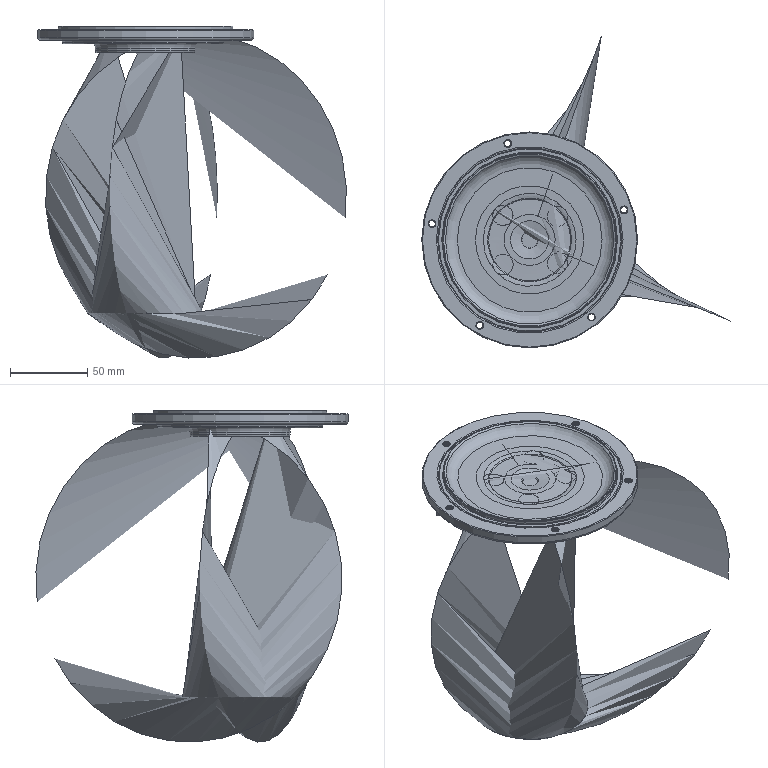NC program | NX | posted with a generic post
Lines 30457 to 31199 of 33119:
(FIXED_CONTOUR_COPY , TOOL : R0.5)
N60900 T02 M6
N60902 G54
N60904 G17 G0 G90 X-60.417 Y-0.5 S9500 M3
N60906 G43 Z30. H2
N60908 Z0.8
N60910 G94 G1 Z-1.85 F1000.
N60912 X-60.416 Y-0.462 Z-2.041
N60914 Y-0.354 Z-2.204
N60916 Y-0.191 Z-2.312
N60918 X-60.415 Y0. Z-2.35
N60920 G2 X-57.918 Y17.189 R60.395 F3500.
N60922 X-52.948 Y29.094 R60.438
N60924 X-28.802 Y53.107 R60.415
N60926 X-17.202 Y57.914 R60.438
N60928 X17.188 Y57.918 R60.415
N60930 X28.789 Y53.115 R60.438
N60932 X53.109 Y28.8 R60.415
N60934 X58.015 Y16.859 R60.438
N60936 X57.917 Y-17.193 R60.415
N60938 X53.109 Y-28.799 R60.438
N60940 X28.807 Y-53.105 R60.415
N60942 X16.865 Y-58.013 R60.438
N60944 X-17.18 Y-57.921 R60.415
N60946 X-29.096 Y-52.947 R60.438
N60948 X-53.105 Y-28.806 R60.415
N60950 X-58.011 Y-16.874 R60.438
N60952 X-60.415 Y0. R60.395
N60954 X34.44 Y49.616 R60.407
N60956 G1 X34.743 Y49.404
N60958 G2 X55.93 Y-22.768 R60.392
N60960 G1 X55.789 Y-23.111 Z-2.351
N60962 G2 X9.994 Y-59.546 R60.382
N60964 G1 X9.628 Y-59.606
N60966 G2 X-35.936 Y-48.513 R60.377
N60968 G1 X-36.234 Y-48.29 Z-2.352
N60970 G2 X-58.454 Y-15.077 R60.369
N60972 G1 X-58.545 Y-14.719
N60974 G2 X-56.71 Y20.677 R60.363
N60976 G1 X-56.583 Y21.024 Z-2.353
N60978 G2 X-34.756 Y49.346 R60.357
N60980 G1 X-34.452 Y49.559
N60982 G2 X-5.546 Y60.098 R60.363
N60984 G1 X-5.178 Y60.131 Z-2.354
N60986 G2 X21.721 Y56.305 R60.344
N60988 G1 X22.066 Y56.171
N60990 G2 X45.946 Y39.123 R60.342
N60992 G1 X46.184 Y38.842 Z-2.355
N60994 G2 X58.047 Y16.483 R60.348
N60996 G1 X58.147 Y16.127
N60998 G2 X59.513 Y-9.951 R60.342
N61000 G1 X59.45 Y-10.317 Z-2.356
N61002 G2 X51.175 Y-31.961 R60.351
N61004 G1 X50.978 Y-32.275
N61006 G2 X35.037 Y-49.116 R60.341
N61008 G1 X34.735 Y-49.33 Z-2.357
N61010 G2 X15.771 Y-58.232 R60.345
N61012 G1 X15.414 Y-58.327
N61014 G2 X-6.655 Y-59.959 R60.328
N61016 G1 X-7.024 Y-59.917 Z-2.358
N61018 G2 X-24.76 Y-55.008 R60.325
N61020 G1 X-25.097 Y-54.856
N61022 G2 X-42.135 Y-43.166 R60.308
N61024 G1 X-42.399 Y-42.907 Z-2.359
N61026 G2 X-53.54 Y-27.783 R60.303
N61028 G1 X-53.708 Y-27.455
N61030 G2 X-59.811 Y-7.795 R60.324
N61032 G1 X-59.857 Y-7.426 Z-2.36
N61034 G2 X-59.291 Y11.06 R60.327
N61036 G1 X-59.222 Y11.423
N61038 G2 X-54.051 Y26.757 R60.325
N61040 G1 X-53.886 Y27.087 Z-2.361
N61042 G2 X-43.417 Y41.858 R60.293
N61044 G1 X-43.159 Y42.124
N61046 G2 X-29.721 Y52.474 R60.292
N61048 G1 X-29.399 Y52.656 Z-2.362
N61050 G2 X-12.87 Y58.915 R60.323
N61052 G1 X-12.507 Y58.993
N61054 G2 X3.341 Y60.21 R60.302
N61056 G1 X3.71 Y60.188 Z-2.363
N61058 G2 X18.568 Y57.37 R60.282
N61060 G1 X18.92 Y57.255
N61062 G2 X34.386 Y49.533 R60.311
N61064 G1 X34.688 Y49.321 Z-2.364
N61066 G2 X45.667 Y39.371 R60.308
N61068 G1 X45.907 Y39.091
N61070 G2 X53.521 Y27.763 R60.276
N61072 G1 X53.69 Y27.435 Z-2.365
N61074 G2 X59.051 Y12.167 R60.307
N61076 G1 X59.125 Y11.805
N61078 G2 X60.261 Y-1.858 R60.286
N61080 G1 X60.249 Y-2.226 Z-2.366
N61082 G2 X58.101 Y-16.09 R60.267
N61084 G1 X58.001 Y-16.446
N61086 G2 X52.639 Y-29.386 R60.307
N61088 G1 X52.458 Y-29.708 Z-2.367
N61090 G2 X44.171 Y-41.025 R60.263
N61092 G1 X43.918 Y-41.296
N61094 G2 X32.87 Y-50.533 R60.277
N61096 G1 X32.559 Y-50.733 Z-2.368
N61098 G2 X22.402 Y-55.963 R60.292
N61100 G1 X22.06 Y-56.099
N61102 G2 X7.035 Y-59.867 R60.274
N61104 G1 X6.665 Y-59.909 Z-2.369
N61106 G2 X-6.28 Y-59.949 R60.304
N61108 G1 X-6.649 Y-59.909
N61110 G2 X-17.847 Y-57.572 R60.259
N61112 G1 X-18.199 Y-57.462 Z-2.37
N61114 G2 X-30.635 Y-51.907 R60.293
N61116 G1 X-30.953 Y-51.718
N61118 G2 X-40.755 Y-44.404 R60.25
N61120 G1 X-41.027 Y-44.152 Z-2.371
N61122 G2 X-49.704 Y-34.087 R60.271
N61124 G1 X-49.912 Y-33.782
N61126 G2 X-54.941 Y-24.775 R60.272
N61128 G1 X-55.091 Y-24.438 Z-2.372
N61130 G2 X-59.239 Y-11.081 R60.276
N61132 G1 X-59.306 Y-10.717
N61134 G2 X-60.265 Y0. R60.254
N61136 G1 X-60.264 Y0.37 Z-2.373
N61138 G2 X-58.876 Y12.86 R60.247
N61140 G1 X-58.796 Y13.22 Z-2.374
N61142 G2 X-55.821 Y22.706 R60.272
N61144 G1 X-55.681 Y23.047
N61146 G2 X-49.079 Y34.966 R60.265
N61148 G1 X-48.863 Y35.267 Z-2.375
N61150 G2 X-42.342 Y42.875 R60.254
N61152 G1 X-42.078 Y43.134
N61154 G2 X-32.546 Y50.712 R60.24
N61156 G1 X-32.234 Y50.911 Z-2.376
N61158 G2 X-24.084 Y55.233 R60.265
N61160 G1 X-23.746 Y55.38
N61162 G2 X-11.043 Y59.234 R60.262
N61164 G1 X-10.678 Y59.3 Z-2.377
N61166 G2 X-1.114 Y60.243 R60.237
N61168 G1 X-0.742 Y60.248
N61170 G2 X11.027 Y59.234 R60.244
N61172 G1 X11.39 Y59.165 Z-2.378
N61174 G2 X19.953 Y56.85 R60.25
N61176 G1 X20.301 Y56.727
N61178 G2 X31.582 Y51.308 R60.265
N61180 G1 X31.895 Y51.113 Z-2.379
N61182 G2 X39.889 Y45.15 R60.224
N61184 G1 X40.167 Y44.903
N61186 G2 X47.723 Y36.77 R60.265
N61188 G1 X47.947 Y36.478 Z-2.38
N61190 G2 X52.781 Y29.043 R60.228
N61192 G1 X52.958 Y28.719
N61194 G2 X56.839 Y19.964 R60.264
N61196 G1 X56.96 Y19.616 Z-2.381
N61198 G2 X59.737 Y7.781 R60.233
N61200 G1 X59.783 Y7.413
N61202 G2 X60.211 Y-1.856 R60.255
N61204 G1 X60.199 Y-2.224 Z-2.382
N61206 G2 X58.853 Y-12.845 R60.217
N61208 G1 X58.773 Y-13.207
N61210 G2 X56.331 Y-21.338 R60.244
N61212 G1 X56.199 Y-21.683 Z-2.383
N61214 G2 X50.893 Y-32.221 R60.249
N61216 G1 X50.694 Y-32.534
N61218 G2 X44.882 Y-40.172 R60.211
N61220 G1 X44.635 Y-40.446 Z-2.384
N61222 G2 X36.469 Y-47.937 R60.25
N61224 G1 X36.174 Y-48.161
N61226 G2 X28.72 Y-52.944 R60.217
N61228 G1 X28.395 Y-53.118 Z-2.385
N61230 G2 X19.271 Y-57.064 R60.251
N61232 G1 X18.921 Y-57.181
N61234 G2 X7.397 Y-59.773 R60.218
N61236 G1 X7.028 Y-59.817 Z-2.386
N61238 G2 X-2.221 Y-60.186 R60.246
N61240 G1 X-2.589 Y-60.172
N61242 G2 X-13.199 Y-58.762 R60.204
N61244 G1 X-13.558 Y-58.68 Z-2.387
N61246 G2 X-21.662 Y-56.194 R60.233
N61248 G1 X-22.005 Y-56.061
N61250 G2 X-32.809 Y-50.501 R60.235
N61252 G1 X-33.119 Y-50.299 Z-2.388
N61254 G2 X-40.721 Y-44.368 R60.2
N61256 G1 X-40.993 Y-44.116
N61258 G2 X-48.595 Y-35.567 R60.229
N61260 G1 X-48.812 Y-35.268 Z-2.389
N61262 G2 X-53.28 Y-28.063 R60.209
N61264 G1 X-53.451 Y-27.736
N61266 G2 X-57.394 Y-18.223 R60.239
N61268 G1 X-57.504 Y-17.871 Z-2.39
N61270 G2 X-59.845 Y-6.674 R60.202
N61272 G1 X-59.885 Y-6.305
N61274 G2 X-60.123 Y3.321 R60.242
N61276 G1 X-60.102 Y3.691 Z-2.391
N61278 G2 X-58.581 Y13.927 R60.19
N61280 G1 X-58.494 Y14.285
N61282 G2 X-55.774 Y22.688 R60.224
N61284 G1 X-55.634 Y23.028 Z-2.392
N61286 G2 X-49.881 Y33.723 R60.218
N61288 G1 X-49.673 Y34.028
N61290 G2 X-43.858 Y41.251 R60.191
N61292 G1 X-43.602 Y41.521 Z-2.393
N61294 G2 X-34.971 Y49.01 R60.209
N61296 G1 X-34.67 Y49.224
N61298 G2 X-27.397 Y53.611 R60.2
N61300 G1 X-27.068 Y53.778 Z-2.394
N61302 G2 X-17.139 Y57.714 R60.226
N61304 G1 X-16.785 Y57.818
N61306 G2 X-5.899 Y59.914 R60.185
N61308 G1 X-5.532 Y59.949 Z-2.395
N61310 G2 X4.439 Y60.038 R60.235
N61312 G1 X4.807 Y60.01
N61314 G2 X14.632 Y58.396 R60.178
N61316 G1 X14.99 Y58.305 Z-2.396
N61318 G2 X23.378 Y55.475 R60.214
N61320 G1 X23.717 Y55.33
N61322 G2 X34.331 Y49.449 R60.202
N61324 G1 X34.633 Y49.238 Z-2.397
N61326 G2 X41.771 Y43.346 R60.183
N61328 G1 X42.038 Y43.086
N61330 G2 X49.427 Y34.357 R60.189
N61332 G1 X49.638 Y34.052 Z-2.398
N61334 G2 X53.933 Y26.731 R60.191
N61336 G1 X54.096 Y26.4
N61338 G2 X58.004 Y16.084 R60.211
N61340 G1 X58.101 Y15.729 Z-2.399
N61342 G2 X59.966 Y5.194 R60.171
N61344 G1 X59.997 Y4.824
N61346 G2 X59.935 Y-5.534 R60.221
N61348 G1 X59.9 Y-5.902 Z-2.4
N61350 G2 X58.198 Y-15.349 R60.168
N61352 G1 X58.103 Y-15.706
N61354 G2 X55.024 Y-24.389 R60.204
N61356 G1 X54.873 Y-24.726 Z-2.401
N61358 G2 X48.776 Y-35.259 R60.185
N61360 G1 X48.559 Y-35.557 Z-2.402
N61362 G2 X42.815 Y-42.296 R60.177
N61364 G1 X42.553 Y-42.56
N61366 G2 X33.738 Y-49.837 R60.172
N61368 G1 X33.432 Y-50.043 Z-2.403
N61370 G2 X26.071 Y-54.241 R60.182
N61372 G1 X25.739 Y-54.399
N61374 G2 X15.015 Y-58.277 R60.197
N61376 G1 X14.657 Y-58.368 Z-2.404
N61378 G2 X4.433 Y-60.015 R60.157
N61380 G1 X4.061 Y-60.041
N61382 G2 X-6.638 Y-59.81 R60.204
N61384 G1 X-7.005 Y-59.768 Z-2.405
N61386 G2 X-16.049 Y-57.996 R60.157
N61388 G1 X-16.404 Y-57.896
N61390 G2 X-25.037 Y-54.718 R60.192
N61392 G1 X-25.371 Y-54.564 Z-2.406
N61394 G2 X-35.821 Y-48.349 R60.169
N61396 G1 X-36.118 Y-48.128
N61398 G2 X-42.814 Y-42.28 R60.171
N61400 G1 X-43.072 Y-42.017 Z-2.407
N61402 G2 X-50.035 Y-33.42 R60.155
N61404 G1 X-50.239 Y-33.113
N61406 G2 X-54.387 Y-25.735 R60.171
N61408 G1 X-54.544 Y-25.402 Z-2.408
N61410 G2 X-58.353 Y-14.663 R60.184
N61412 G1 X-58.442 Y-14.305
N61414 G2 X-60.027 Y-4.078 R60.144
N61416 G1 X-60.051 Y-3.707 Z-2.409
N61418 G2 X-59.754 Y7.012 R60.189
N61420 G1 X-59.71 Y7.38
N61422 G2 X-57.882 Y16.409 R60.146
N61424 G1 X-57.781 Y16.763 Z-2.41
N61426 G2 X-54.396 Y25.7 R60.181
N61428 G1 X-54.238 Y26.032
N61430 G2 X-47.899 Y36.4 R60.154
N61432 G1 X-47.674 Y36.694 Z-2.411
N61434 G2 X-41.479 Y43.572 R60.168
N61436 G1 X-41.212 Y43.825
N61438 G2 X-32.493 Y50.627 R60.138
N61440 G1 X-32.181 Y50.826 Z-2.412
N61442 G2 X-24.718 Y54.843 R60.163
N61444 G1 X-24.381 Y54.994
N61446 G2 X-13.196 Y58.689 R60.167
N61448 G1 X-12.836 Y58.769 Z-2.413
N61450 G2 X-3.325 Y60.061 R60.131
N61452 G1 X-2.957 Y60.08
N61454 G2 X8.097 Y59.604 R60.167
N61456 G1 X8.462 Y59.554 Z-2.414
N61458 G2 X17.112 Y57.665 R60.137
N61460 G1 X17.466 Y57.559
N61462 G2 X26.706 Y53.895 R60.169
N61464 G1 X27.035 Y53.731 Z-2.415
N61466 G2 X36.977 Y47.439 R60.137
N61468 G1 X37.268 Y47.211
N61470 G2 X44.078 Y40.924 R60.164
N61472 G1 X44.328 Y40.652 Z-2.416
N61474 G2 X50.817 Y32.173 R60.124
N61476 G1 X51.013 Y31.86
N61478 G2 X55.131 Y24.037 R60.152
N61480 G1 X55.277 Y23.7 Z-2.417
N61482 G2 X58.83 Y12.493 R60.152
N61484 G1 X58.906 Y12.132
N61486 G2 X60.085 Y2.595 R60.121
N61488 G1 X60.099 Y2.223 Z-2.418
N61490 G2 X59.488 Y-8.823 R60.148
N61492 G1 X59.433 Y-9.188
N61494 G2 X57.438 Y-17.818 R60.128
N61496 G1 X57.327 Y-18.17 Z-2.419
N61498 G2 X53.382 Y-27.69 R60.156
N61500 G1 X53.211 Y-28.017
N61502 G2 X46.95 Y-37.575 R60.121
N61504 G1 X46.719 Y-37.862 Z-2.42
N61506 G2 X40.105 Y-44.807 R60.161
N61508 G1 X39.83 Y-45.051
N61510 G2 X31.543 Y-51.195 R60.111
N61512 G1 X31.228 Y-51.387 Z-2.421
N61514 G2 X23.366 Y-55.405 R60.142
N61516 G1 X23.026 Y-55.547
N61518 G2 X11.401 Y-59.039 R60.136
N61520 G1 X11.038 Y-59.107 Z-2.422
N61522 G2 X1.835 Y-60.1 R60.111
N61524 G1 X1.466 Y-60.11
N61526 G2 X-9.922 Y-59.302 R60.128
N61528 G1 X-10.286 Y-59.24 Z-2.423
N61530 G2 X-18.505 Y-57.207 R60.119
N61532 G1 X-18.855 Y-57.092
N61534 G2 X-28.639 Y-52.865 R60.143
N61536 G1 X-28.963 Y-52.688 Z-2.424
N61538 G2 X-38.129 Y-46.485 R60.106
N61540 G1 X-38.415 Y-46.249
N61542 G2 X-45.523 Y-39.271 R60.151
N61544 G1 X-45.763 Y-38.991 Z-2.425
N61546 G2 X-51.569 Y-30.903 R60.098
N61548 G1 X-51.757 Y-30.587
N61550 G2 X-55.674 Y-22.684 R60.132
N61552 G1 X-55.812 Y-22.343 Z-2.426
N61554 G2 X-59.16 Y-10.684 R60.121
N61556 G1 X-59.224 Y-10.321
N61558 G2 X-60.105 Y-1.104 R60.102
N61560 G1 X-60.111 Y-0.736 Z-2.427
N61562 G2 X-59.162 Y10.657 R60.109
N61564 G1 X-59.095 Y11.02
N61566 G2 X-56.962 Y19.205 R60.11
N61568 G1 X-56.844 Y19.553 Z-2.428
N61570 G2 X-52.499 Y29.277 R60.13
N61572 G1 X-52.319 Y29.598
N61574 G2 X-46.245 Y38.4 R60.092
N61576 G1 X-46.007 Y38.685 Z-2.429
N61578 G2 X-38.699 Y45.994 R60.138
N61580 G1 X-38.416 Y46.23 Z-2.43
N61582 G2 X-30.581 Y51.746 R60.087
N61584 G1 X-30.263 Y51.933
N61586 G2 X-21.983 Y55.941 R60.121
N61588 G1 X-21.64 Y56.075 Z-2.431
N61590 G2 X-9.922 Y59.28 R60.105
N61592 G1 X-9.557 Y59.34
N61594 G2 X-0.74 Y60.098 R60.093
N61596 G1 X-0.369 Y60.102 Z-2.432
N61598 G2 X10.999 Y59.086 R60.093
N61600 G1 X11.362 Y59.018
N61602 G2 X19.555 Y56.83 R60.099
N61604 G1 X19.903 Y56.709 Z-2.433
N61606 G2 X29.926 Y52.118 R60.116
N61608 G1 X30.244 Y51.934
N61610 G2 X38.953 Y45.764 R60.078
N61612 G1 X39.234 Y45.523 Z-2.434
N61614 G2 X46.693 Y37.833 R60.122
N61616 G1 X46.923 Y37.546
N61618 G2 X52.108 Y29.936 R60.077
N61620 G1 X52.29 Y29.615 Z-2.435
N61622 G2 X56.194 Y21.293 R60.109
N61624 G1 X56.323 Y20.949
N61626 G2 X59.38 Y9.219 R60.09
N61628 G1 X59.436 Y8.854 Z-2.436
N61630 G2 X60.089 Y-0.378 R60.089
N61632 G1 X60.086 Y-0.747
N61634 G2 X58.933 Y-11.728 R60.075
N61636 G1 X58.86 Y-12.09 Z-2.437
N61638 G2 X56.573 Y-20.248 R60.089
N61640 G1 X56.448 Y-20.594
N61642 G2 X51.541 Y-30.885 R60.101
N61644 G1 X51.35 Y-31.201 Z-2.438
N61646 G2 X45.258 Y-39.52 R60.064
N61648 G1 X45.015 Y-39.797
N61650 G2 X37.255 Y-47.139 R60.106
N61652 G1 X36.964 Y-47.367 Z-2.439
N61654 G2 X29.293 Y-52.457 R60.066
N61656 G1 X28.971 Y-52.635
N61658 G2 X20.262 Y-56.561 R60.098
N61660 G1 X19.915 Y-56.684 Z-2.44
N61662 G2 X8.476 Y-59.478 R60.074
N61664 G1 X8.11 Y-59.529
N61666 G2 X-1.113 Y-60.067 R60.083
N61668 G1 X-1.48 Y-60.059 Z-2.441
N61670 G2 X-12.446 Y-58.773 R60.059
N61672 G1 X-12.806 Y-58.695
N61674 G2 X-21.266 Y-56.185 R60.081
N61676 G1 X-21.609 Y-56.054 Z-2.442
N61678 G2 X-32.111 Y-50.771 R60.085
N61680 G1 X-32.422 Y-50.573
N61682 G2 X-40.07 Y-44.756 R60.052
N61684 G1 X-40.345 Y-44.507 Z-2.443
N61686 G2 X-47.811 Y-36.367 R60.086
N61688 G1 X-48.034 Y-36.073
N61690 G2 X-52.801 Y-28.641 R60.057
N61692 G1 X-52.976 Y-28.318 Z-2.444
N61694 G2 X-56.91 Y-19.221 R60.086
N61696 G1 X-57.026 Y-18.873
N61698 G2 X-59.61 Y-7.387 R60.057
N61700 G1 X-59.655 Y-7.02 Z-2.445
N61702 G2 X-60.01 Y2.577 R60.083
N61704 G1 X-59.993 Y2.945
N61706 G2 X-58.519 Y13.532 R60.044
N61708 G1 X-58.435 Y13.89 Z-2.446
N61710 G2 X-55.772 Y22.292 R60.072
N61712 G1 X-55.635 Y22.633
N61714 G2 X-50.163 Y33.03 R60.069
N61716 G1 X-49.959 Y33.337 Z-2.447
N61718 G2 X-44.002 Y40.877 R60.042
N61720 G1 X-43.749 Y41.148
N61722 G2 X-35.482 Y48.456 R60.063
N61724 G1 X-35.184 Y48.673 Z-2.448
N61726 G2 X-27.657 Y53.309 R60.049
N61728 G1 X-27.329 Y53.478
N61730 G2 X-17.799 Y57.357 R60.074
N61732 G1 X-17.447 Y57.465 Z-2.449
N61734 G2 X-6.251 Y59.728 R60.04
N61736 G1 X-5.885 Y59.765
N61738 G2 X4.06 Y59.915 R60.08
N61740 G1 X4.427 Y59.889 Z-2.45
N61742 G2 X14.237 Y58.339 R60.031
N61744 G1 X14.595 Y58.25
N61746 G2 X22.98 Y55.479 R60.062
N61748 G1 X23.32 Y55.337 Z-2.451
N61750 G2 X33.642 Y49.739 R60.053
N61752 G1 X33.946 Y49.532
N61754 G2 X41.129 Y43.749 R60.031
N61756 G1 X41.399 Y43.494 Z-2.452
N61758 G2 X48.664 Y35.175 R60.047
N61760 G1 X48.879 Y34.875
N61762 G2 X53.468 Y27.322 R60.038
N61764 G1 X53.634 Y26.994 Z-2.453
N61766 G2 X57.451 Y17.451 R60.06
N61768 G1 X57.556 Y17.099
N61770 G2 X59.712 Y6.282 R60.027
N61772 G1 X59.749 Y5.914 Z-2.454
N61774 G2 X59.903 Y-4.05 R60.065
N61776 G1 X59.877 Y-4.417
N61778 G2 X58.326 Y-14.238 R60.019
N61780 G1 X58.237 Y-14.596 Z-2.455
N61782 G2 X55.467 Y-22.976 R60.049
N61784 G1 X55.325 Y-23.316
N61786 G2 X49.713 Y-33.659 R60.041
N61788 G1 X49.505 Y-33.964 Z-2.456
N61790 G2 X43.735 Y-41.126 R60.018
N61792 G1 X43.481 Y-41.394
N61794 G2 X35.164 Y-48.657 R60.035
N61796 G1 X34.864 Y-48.872 Z-2.457
N61798 G2 X27.323 Y-53.453 R60.025
N61800 G1 X26.995 Y-53.62
N61802 G2 X17.452 Y-57.437 R60.048
N61804 G1 X17.1 Y-57.543 Z-2.458
N61806 G2 X6.266 Y-59.701 R60.015
N61808 G1 X5.897 Y-59.738
N61810 G2 X-4.048 Y-59.891 R60.053
N61812 G1 X-4.415 Y-59.865 Z-2.459
N61814 G2 X-14.229 Y-58.315 R60.006
N61816 G1 X-14.586 Y-58.227 Z-2.46
N61818 G2 X-22.956 Y-55.461 R60.036
N61820 G1 X-23.295 Y-55.32
N61822 G2 X-33.627 Y-49.719 R60.029
N61824 G1 X-33.932 Y-49.512 Z-2.461
N61826 G2 X-41.126 Y-43.719 R60.006
N61828 G1 X-41.393 Y-43.465
N61830 G2 X-48.649 Y-35.152 R60.023
N61832 G1 X-48.864 Y-34.853 Z-2.462
N61834 G2 X-53.442 Y-27.317 R60.013
N61836 G1 X-53.608 Y-26.99
N61838 G2 X-57.423 Y-17.455 R60.035
N61840 G1 X-57.529 Y-17.103 Z-2.463
N61842 G2 X-59.687 Y-6.278 R60.003
N61844 G1 X-59.725 Y-5.91
N61846 G2 X-59.878 Y4.049 R60.04
N61848 G1 X-59.852 Y4.418 Z-2.464
N61850 G2 X-58.301 Y14.236 R59.994
N61852 G1 X-58.212 Y14.592
N61854 G2 X-55.449 Y22.954 R60.024
N61856 G1 X-55.307 Y23.293 Z-2.465
N61858 G2 X-49.711 Y33.616 R60.016
N61860 G1 X-49.504 Y33.921
N61862 G2 X-43.712 Y41.114 R59.994
N61864 G1 X-43.458 Y41.382 Z-2.466
N61866 G2 X-35.154 Y48.633 R60.01
N61868 G1 X-34.855 Y48.847
N61870 G2 X-27.307 Y53.433 R60.001
N61872 G1 X-26.979 Y53.6 Z-2.467
N61874 G2 X-17.432 Y57.417 R60.023
N61876 G1 X-17.08 Y57.523
N61878 G2 X-6.246 Y59.678 R59.99
N61880 G1 X-5.88 Y59.715 Z-2.468
N61882 G2 X4.056 Y59.865 R60.028
N61884 G1 X4.423 Y59.839
N61886 G2 X14.225 Y58.29 R59.982
N61888 G1 X14.582 Y58.202 Z-2.469
N61890 G2 X23.3 Y55.291 R60.011
N61892 G1 X23.639 Y55.147
N61894 G2 X33.919 Y49.49 R60.002
N61896 G1 X34.222 Y49.281 Z-2.47
N61898 G2 X41.365 Y43.458 R59.984
N61900 G1 X41.633 Y43.201
N61902 G2 X48.838 Y34.846 R59.994
N61904 G1 X49.052 Y34.546 Z-2.471
N61906 G2 X53.589 Y26.971 R59.99
N61908 G1 X53.754 Y26.643
N61910 G2 X57.612 Y16.732 R60.009
N61912 G1 X57.713 Y16.379 Z-2.472
N61914 G2 X59.735 Y5.54 R59.976
N61916 G1 X59.768 Y5.172
N61918 G2 X59.768 Y-5.148 R60.016
N61920 G1 X59.736 Y-5.515 Z-2.473
N61922 G2 X58.098 Y-14.941 R59.971
N61924 G1 X58.005 Y-15.297
N61926 G2 X54.989 Y-23.972 R60.
N61928 G1 X54.841 Y-24.309 Z-2.474
N61930 G2 X49.043 Y-34.541 R59.987
N61932 G1 X48.829 Y-34.842
N61934 G2 X42.932 Y-41.892 R59.975
N61936 G1 X42.673 Y-42.156 Z-2.475
N61938 G2 X34.234 Y-49.255 R59.976
N61940 G1 X33.931 Y-49.464
N61942 G2 X26.314 Y-53.901 R59.98
N61944 G1 X25.984 Y-54.061 Z-2.476
N61946 G2 X15.67 Y-57.897 R59.995
N61948 G1 X15.315 Y-57.992
N61950 G2 X4.786 Y-59.787 R59.962
N61952 G1 X4.417 Y-59.816 Z-2.477
N61954 G2 X-5.881 Y-59.688 R60.002
N61956 G1 X-6.248 Y-59.651
N61958 G2 X-15.641 Y-57.9 R59.96
N61960 G1 X-15.996 Y-57.803 Z-2.478
N61962 G2 X-24.957 Y-54.535 R59.989
N61964 G1 X-25.291 Y-54.381
N61966 G2 X-35.409 Y-48.404 R59.971
N61968 G1 X-35.706 Y-48.185 Z-2.479
N61970 G2 X-42.671 Y-42.14 R59.969
N61972 G1 X-42.928 Y-41.878
N61974 G2 X-49.868 Y-33.311 R59.958
N61976 G1 X-50.071 Y-33.004 Z-2.48
N61978 G2 X-54.363 Y-25.315 R59.971
N61980 G1 X-54.517 Y-24.982
N61982 G2 X-58.161 Y-14.607 R59.981
N61984 G1 X-58.25 Y-14.25 Z-2.481
N61986 G2 X-59.828 Y-4.061 R59.949
N61988 G1 X-59.852 Y-3.692
N61990 G2 X-59.556 Y6.987 R59.985
N61992 G1 X-59.512 Y7.353 Z-2.482
N61994 G2 X-57.69 Y16.353 R59.949
N61996 G1 X-57.589 Y16.706
N61998 G2 X-54.214 Y25.619 R59.978
N62000 G1 X-54.056 Y25.95 Z-2.483
N62002 G2 X-47.958 Y35.99 R59.956
N62004 G1 X-47.736 Y36.284
N62006 G2 X-41.607 Y43.174 R59.963
N62008 G1 X-41.342 Y43.427 Z-2.484
N62010 G2 X-32.695 Y50.259 R59.943
N62012 G1 X-32.385 Y50.459
N62014 G2 X-24.635 Y54.661 R59.961
N62016 G1 X-24.3 Y54.811 Z-2.485
N62018 G2 X-13.509 Y58.413 R59.966
N62020 G1 X-13.15 Y58.495
N62022 G2 X-3.313 Y59.862 R59.935
N62024 G1 X-2.946 Y59.881 Z-2.486
N62026 G2 X8.07 Y59.406 R59.965
N62028 G1 X8.434 Y59.356
N62030 G2 X17.407 Y57.368 R59.94
N62032 G1 X17.758 Y57.26 Z-2.487
N62034 G2 X26.947 Y53.552 R59.966
N62036 G1 X27.274 Y53.386
N62038 G2 X36.859 Y47.277 R59.939
N62040 G1 X37.149 Y47.05 Z-2.488
N62042 G2 X44.179 Y40.519 R59.963
N62044 G1 X44.427 Y40.247
N62046 G2 X50.647 Y32.066 R59.928
N62048 G1 X50.843 Y31.755 Z-2.489
N62050 G2 X54.948 Y23.957 R59.951
N62052 G1 X55.094 Y23.62 Z-2.49
N62054 G2 X58.559 Y12.804 R59.951
N62056 G1 X58.636 Y12.445
N62058 G2 X59.868 Y2.954 R59.924
N62060 G1 X59.885 Y2.584 Z-2.491
N62062 G2 X59.344 Y-8.43 R59.95
N62064 G1 X59.291 Y-8.794
N62066 G2 X57.355 Y-17.406 R59.929
N62068 G1 X57.247 Y-17.757 Z-2.492
N62070 G2 X53.539 Y-26.945 R59.953
N62072 G1 X53.372 Y-27.272
N62074 G2 X47.249 Y-36.875 R59.926
N62076 G1 X47.022 Y-37.163 Z-2.493
N62078 G2 X40.517 Y-44.164 R59.951
N62080 G1 X40.245 Y-44.412
N62082 G2 X32.062 Y-50.636 R59.915
N62084 G1 X31.751 Y-50.831 Z-2.494
N62086 G2 X23.96 Y-54.933 R59.938
N62088 G1 X23.623 Y-55.079
N62090 G2 X12.799 Y-58.547 R59.939
N62092 G1 X12.44 Y-58.624 Z-2.495
N62094 G2 X2.936 Y-59.856 R59.911
N62096 G1 X2.567 Y-59.873
N62098 G2 X-8.435 Y-59.33 R59.937
N62100 G1 X-8.799 Y-59.277 Z-2.496
N62102 G2 X-17.744 Y-57.238 R59.917
N62104 G1 X-18.095 Y-57.128
N62106 G2 X-27.576 Y-53.202 R59.94
N62108 G1 X-27.901 Y-53.032 Z-2.497
N62110 G2 X-37.142 Y-47.024 R59.912
N62112 G1 X-37.431 Y-46.794
N62114 G2 X-44.399 Y-40.241 R59.94
N62116 G1 X-44.644 Y-39.968 Z-2.498
N62118 G2 X-50.822 Y-31.741 R59.903
N62120 G1 X-51.016 Y-31.429
N62122 G2 X-55.067 Y-23.62 R59.927
N62124 G1 X-55.21 Y-23.283 Z-2.499
N62126 G2 X-58.61 Y-12.446 R59.925
N62128 G1 X-58.686 Y-12.086
N62130 G2 X-59.86 Y-2.579 R59.9
N62132 G1 X-59.875 Y-2.209 Z-2.5
N62134 G2 X-59.264 Y8.805 R59.922
N62136 G1 X-59.209 Y9.169
N62138 G2 X-57.225 Y17.746 R59.905
N62140 G1 X-57.115 Y18.096 Z-2.501
N62142 G2 X-53.191 Y27.57 R59.927
N62144 G1 X-53.021 Y27.895
N62146 G2 X-47.018 Y37.129 R59.9
N62148 G1 X-46.788 Y37.418 Z-2.502
N62150 G2 X-40.233 Y44.389 R59.927
N62152 G1 X-39.96 Y44.635
N62154 G2 X-31.737 Y50.81 R59.89
N62156 G1 X-31.424 Y51.004 Z-2.503
N62158 G2 X-23.269 Y55.202 R59.915
N62160 G1 X-22.93 Y55.344
N62162 G2 X-11.698 Y58.751 R59.911
N62164 G1 X-11.337 Y58.822 Z-2.504
N62166 G2 X-1.842 Y59.875 R59.889
N62168 G1 X-1.474 Y59.885
N62170 G2 X9.515 Y59.141 R59.903
N62172 G1 X9.878 Y59.082 Z-2.505
N62174 G2 X18.444 Y56.99 R59.895
N62176 G1 X18.793 Y56.876
N62178 G2 X28.226 Y52.831 R59.915
N62180 G1 X28.549 Y52.658 Z-2.506
N62182 G2 X37.694 Y46.55 R59.885
N62184 G1 X37.979 Y46.317
N62186 G2 X45.121 Y39.391 R59.919
N62188 G1 X45.361 Y39.114 Z-2.507
N62190 G2 X51.186 Y31.103 R59.878
N62192 G1 X51.376 Y30.788
N62194 G2 X55.472 Y22.585 R59.904
N62196 G1 X55.609 Y22.245 Z-2.508
N62198 G2 X58.875 Y10.993 R59.896
N62200 G1 X58.941 Y10.632
N62202 G2 X59.873 Y1.472 R59.879
N62204 G1 X59.88 Y1.102 Z-2.509
N62206 G2 X59.069 Y-9.877 R59.888
N62208 G1 X59.007 Y-10.24
N62210 G2 X56.863 Y-18.791 R59.884
N62212 G1 X56.747 Y-19.14 Z-2.51
N62214 G2 X52.467 Y-28.872 R59.902
N62216 G1 X52.289 Y-29.193
N62218 G2 X46.293 Y-37.989 R59.871
N62220 G1 X46.059 Y-38.272 Z-2.511
N62222 G2 X39.113 Y-45.346 R59.908
N62224 G1 X38.834 Y-45.585
N62226 G2 X30.785 Y-51.363 R59.866
N62228 G1 X30.469 Y-51.551 Z-2.512
N62230 G2 X22.248 Y-55.595 R59.892
N62232 G1 X21.907 Y-55.73
N62234 G2 X10.624 Y-58.93 R59.882
N62236 G1 X10.261 Y-58.994 Z-2.513
N62238 G2 X1.095 Y-59.868 R59.867
N62240 G1 X0.727 Y-59.874
N62242 G2 X-10.242 Y-58.994 R59.874
N62244 G1 X-10.603 Y-58.93 Z-2.514
N62246 G2 X-19.126 Y-56.739 R59.873
N62248 G1 X-19.473 Y-56.62
N62250 G2 X-29.169 Y-52.288 R59.888
N62252 G1 X-29.489 Y-52.108 Z-2.515
N62254 G2 X-38.258 Y-46.055 R59.859
N62256 G1 X-38.541 Y-45.818
N62258 G2 X-45.811 Y-38.547 R59.895
N62260 G1 X-46.047 Y-38.265 Z-2.516
N62262 G2 X-51.727 Y-30.144 R59.854
N62264 G1 X-51.911 Y-29.827
N62266 G2 X-55.981 Y-21.222 R59.881
N62268 G1 X-56.11 Y-20.879 Z-2.517
N62270 G2 X-59.101 Y-9.543 R59.866
N62272 G1 X-59.159 Y-9.18
N62274 G2 X-59.865 Y0. R59.861
N62276 G1 X-59.864 Y0.367 Z-2.518
N62278 G2 X-58.782 Y11.331 R59.855
N62280 G1 X-58.711 Y11.692
N62282 G2 X-56.365 Y20.164 R59.864
N62284 G1 X-56.24 Y20.509 Z-2.519
N62286 G2 X-51.547 Y30.435 R59.874
N62288 G1 X-51.36 Y30.75
N62290 G2 X-45.335 Y39.089 R59.845
N62292 G1 X-45.093 Y39.368 Z-2.52
N62294 G2 X-37.403 Y46.734 R59.878
N62296 G1 X-37.116 Y46.962
N62298 G2 X-29.181 Y52.262 R59.845
N62300 G1 X-28.86 Y52.44 Z-2.521
N62302 G2 X-20.173 Y56.354 R59.87
N62304 G1 X-19.828 Y56.476 Z-2.522
N62306 G2 X-8.787 Y59.206 R59.851
N62308 G1 X-8.423 Y59.259
N62310 G2 X0.739 Y59.848 R59.855
N62312 G1 X1.107 Y59.843 Z-2.523
N62314 G2 X12.036 Y58.629 R59.839
N62316 G1 X12.396 Y58.554
N62318 G2 X20.855 Y56.099 R59.854
N62320 G1 X21.198 Y55.97 Z-2.524
N62322 G2 X31.067 Y51.154 R59.859
N62324 G1 X31.38 Y50.963
N62326 G2 X39.354 Y45.089 R59.832
N62328 G1 X39.631 Y44.845 Z-2.525
N62330 G2 X46.955 Y37.105 R59.863
N62332 G1 X47.181 Y36.817
N62334 G2 X52.252 Y29.173 R59.833
N62336 G1 X52.43 Y28.852 Z-2.526
N62338 G2 X56.341 Y20.171 R59.857
N62340 G1 X56.464 Y19.826
N62342 G2 X59.19 Y8.809 R59.838
N62344 G1 X59.243 Y8.445 Z-2.527
N62346 G2 X59.836 Y-0.742 R59.842
N62348 G1 X59.83 Y-1.109
N62350 G2 X58.616 Y-12.038 R59.827
N62352 G1 X58.54 Y-12.398 Z-2.528
N62354 G2 X56.087 Y-20.852 R59.841
N62356 G1 X55.958 Y-21.195
N62358 G2 X51.136 Y-31.073 R59.847
N62360 G1 X50.944 Y-31.386 Z-2.529
N62362 G2 X45.069 Y-39.357 R59.819
N62364 G1 X44.827 Y-39.632
N62366 G2 X37.1 Y-46.943 R59.851
N62368 G1 X36.811 Y-47.17 Z-2.53
N62370 G2 X29.171 Y-52.239 R59.82
N62372 G1 X28.851 Y-52.417
N62374 G2 X20.173 Y-56.327 R59.844
N62376 G1 X19.828 Y-56.45 Z-2.531
N62378 G2 X8.799 Y-59.179 R59.826